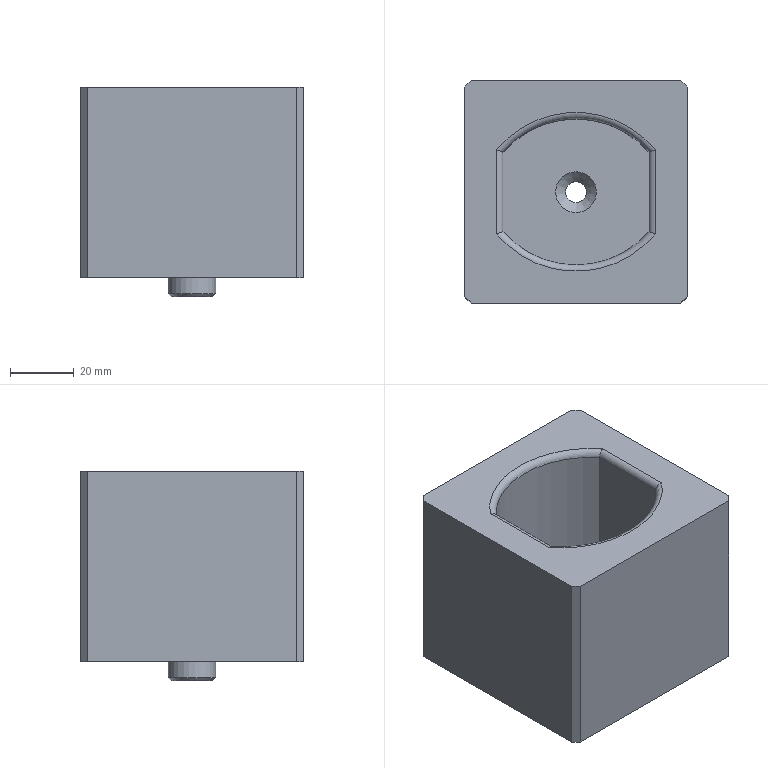NC program | NX | posted with a generic post | part box 70 x 70 x 66 mm
Lines 6381 to 7171 of 8582:
(ZLEVEL_PROFILE_COPY_1_COPY_COPY , TOOL : D6R3)
N12724 T23 M6
N12726 G54
N12728 G17 G0 G90 X-1.4 Y24.719 S7500 M3
N12730 G43 Z30. H23
N12732 Z1.4
N12734 G94 G1 X-3.287 Y24.591 Z1.301 F1000.
N12736 X-5.461 Y24.292 Z1.186
N12738 X-7.61 Y23.847 Z1.071
N12740 X-9.723 Y23.256 Z0.956
N12742 X-11.792 Y22.522 Z0.841
N12744 X-13.805 Y21.649 Z0.726
N12746 X-15.755 Y20.641 Z0.611
N12748 X-17.631 Y19.503 Z0.496
N12750 X-19.425 Y18.239 Z0.381
N12752 X-21.129 Y16.856 Z0.266
N12754 X-22.735 Y15.361 Z0.151
N12756 X-24.236 Y13.759 Z0.036
N12758 X-24.749 Y13.142 Z-0.006
N12760 Y-13.142 F2500.
N12762 G3 X24.749 Y-13.142 R32.189
N12764 G1 Y13.142
N12766 G3 X-24.749 Y13.142 R32.189
N12768 G1 X-24.714 Y13.035 Z-0.008
N12770 X-24.684 Y12.93 Z-0.01
N12772 X-24.656 Y12.824 Z-0.012
N12774 X-24.63 Y12.718 Z-0.014
N12776 Y-13.099
N12778 G3 X24.63 Y-13.099 R32.07
N12780 G1 Y13.099
N12782 G3 X-24.63 Y13.099 R32.07
N12784 G1 X-24.599 Y12.962 Z-0.016
N12786 X-24.57 Y12.826 Z-0.018
N12788 X-24.544 Y12.69 Z-0.021
N12790 X-24.518 Y12.553 Z-0.023
N12792 Y-13.059
N12794 G3 X24.518 Y-13.059 R31.959
N12796 G1 Y13.059
N12798 G3 X-24.518 Y13.059 R31.959
N12800 G1 X-24.489 Y12.893 Z-0.026
N12802 X-24.462 Y12.727 Z-0.029
N12804 X-24.436 Y12.561 Z-0.032
N12806 X-24.411 Y12.395 Z-0.035
N12808 Y-13.02
N12810 G3 X24.411 Y-13.02 R31.851
N12812 G1 Y13.02
N12814 G3 X-24.411 Y13.02 R31.851
N12816 G1 X-24.392 Y12.891 Z-0.037
N12818 X-24.374 Y12.762 Z-0.039
N12820 X-24.356 Y12.633 Z-0.042
N12822 X-24.339 Y12.504 Z-0.044
N12824 X-24.323 Y12.375 Z-0.046
N12826 X-24.306 Y12.246 Z-0.048
N12828 Y-12.982
N12830 G3 X24.306 Y-12.982 R31.747
N12832 G1 Y12.982
N12834 G3 X-24.306 Y12.982 R31.747
N12836 G1 X-24.288 Y12.833 Z-0.051
N12838 X-24.27 Y12.684 Z-0.054
N12840 X-24.253 Y12.535 Z-0.056
N12842 X-24.236 Y12.387 Z-0.059
N12844 X-24.219 Y12.238 Z-0.061
N12846 X-24.203 Y12.089 Z-0.064
N12848 Y-12.944
N12850 G3 X24.203 Y-12.944 R31.644
N12852 G1 Y12.944
N12854 G3 X-24.203 Y12.944 R31.644
N12856 G1 X-24.185 Y12.777 Z-0.067
N12858 X-24.168 Y12.61 Z-0.07
N12860 X-24.151 Y12.443 Z-0.073
N12862 X-24.134 Y12.276 Z-0.076
N12864 X-24.118 Y12.109 Z-0.078
N12866 X-24.102 Y11.943 Z-0.081
N12868 Y-12.907
N12870 G3 X24.102 Y-12.907 R31.542
N12872 G1 Y12.907
N12874 G3 X-24.102 Y12.907 R31.542
N12876 G1 X-24.088 Y12.767 Z-0.084
N12878 X-24.075 Y12.628 Z-0.086
N12880 X-24.062 Y12.488 Z-0.089
N12882 X-24.05 Y12.349 Z-0.091
N12884 X-24.037 Y12.209 Z-0.094
N12886 X-24.025 Y12.07 Z-0.096
N12888 X-24.013 Y11.93 Z-0.098
N12890 X-24.001 Y11.791 Z-0.101
N12892 Y-12.87
N12894 G3 X24.001 Y-12.87 R31.441
N12896 G1 Y12.87
N12898 G3 X-24.001 Y12.87 R31.441
N12900 G1 X-23.988 Y12.716 Z-0.104
N12902 X-23.975 Y12.563 Z-0.106
N12904 X-23.962 Y12.409 Z-0.109
N12906 X-23.95 Y12.255 Z-0.112
N12908 X-23.937 Y12.101 Z-0.114
N12910 X-23.925 Y11.948 Z-0.117
N12912 X-23.913 Y11.794 Z-0.12
N12914 X-23.901 Y11.64 Z-0.122
N12916 Y-12.833
N12918 G3 X23.901 Y-12.833 R31.341
N12920 G1 Y12.833
N12922 G3 X-23.901 Y12.833 R31.341
N12924 G1 X-23.888 Y12.666 Z-0.125
N12926 X-23.875 Y12.498 Z-0.128
N12928 X-23.863 Y12.331 Z-0.131
N12930 X-23.85 Y12.163 Z-0.134
N12932 X-23.838 Y11.995 Z-0.137
N12934 X-23.826 Y11.828 Z-0.14
N12936 X-23.814 Y11.66 Z-0.143
N12938 X-23.802 Y11.493 Z-0.146
N12940 Y-12.797
N12942 G3 X23.802 Y-12.797 R31.242
N12944 G1 Y12.797
N12946 G3 X-23.802 Y12.797 R31.242
N12948 G1 X-23.791 Y12.652 Z-0.148
N12950 X-23.781 Y12.507 Z-0.151
N12952 X-23.771 Y12.362 Z-0.153
N12954 X-23.761 Y12.217 Z-0.156
N12956 X-23.751 Y12.072 Z-0.158
N12958 X-23.742 Y11.927 Z-0.161
N12960 X-23.732 Y11.782 Z-0.163
N12962 X-23.722 Y11.637 Z-0.166
N12964 X-23.713 Y11.492 Z-0.169
N12966 X-23.703 Y11.347 Z-0.171
N12968 Y-12.761
N12970 G3 X23.703 Y-12.761 R31.144
N12972 G1 Y12.761
N12974 G3 X-23.703 Y12.761 R31.144
N12976 G1 X-23.693 Y12.605 Z-0.174
N12978 X-23.683 Y12.448 Z-0.176
N12980 X-23.673 Y12.292 Z-0.179
N12982 X-23.663 Y12.136 Z-0.182
N12984 X-23.654 Y11.98 Z-0.185
N12986 X-23.644 Y11.824 Z-0.187
N12988 X-23.634 Y11.667 Z-0.19
N12990 X-23.625 Y11.511 Z-0.193
N12992 X-23.615 Y11.355 Z-0.196
N12994 X-23.606 Y11.199 Z-0.198
N12996 Y-12.725
N12998 G3 X23.606 Y-12.725 R31.046
N13000 G1 Y12.725
N13002 G3 X-23.606 Y12.725 R31.046
N13004 G1 X-23.596 Y12.558 Z-0.201
N13006 X-23.586 Y12.39 Z-0.204
N13008 X-23.576 Y12.223 Z-0.207
N13010 X-23.566 Y12.056 Z-0.21
N13012 X-23.557 Y11.889 Z-0.213
N13014 X-23.547 Y11.722 Z-0.216
N13016 X-23.537 Y11.554 Z-0.219
N13018 X-23.528 Y11.387 Z-0.222
N13020 X-23.518 Y11.22 Z-0.225
N13022 X-23.509 Y11.053 Z-0.227
N13024 Y-12.689
N13026 G3 X23.509 Y-12.689 R30.949
N13028 G1 Y12.689
N13030 G3 X-23.509 Y12.689 R30.949
N13032 G1 X-23.501 Y12.541 Z-0.23
N13034 X-23.492 Y12.392 Z-0.233
N13036 X-23.484 Y12.244 Z-0.235
N13038 X-23.476 Y12.095 Z-0.238
N13040 X-23.468 Y11.947 Z-0.24
N13042 X-23.46 Y11.799 Z-0.243
N13044 X-23.452 Y11.65 Z-0.246
N13046 X-23.444 Y11.502 Z-0.248
N13048 X-23.436 Y11.354 Z-0.251
N13050 X-23.428 Y11.205 Z-0.253
N13052 X-23.421 Y11.057 Z-0.256
N13054 X-23.413 Y10.908 Z-0.259
N13056 Y-12.653
N13058 G3 X23.413 Y-12.653 R30.853
N13060 G1 Y12.653
N13062 G3 X-23.413 Y12.653 R30.853
N13064 G1 X-23.405 Y12.496 Z-0.261
N13066 X-23.397 Y12.338 Z-0.264
N13068 X-23.388 Y12.181 Z-0.267
N13070 X-23.38 Y12.023 Z-0.27
N13072 X-23.372 Y11.866 Z-0.272
N13074 X-23.364 Y11.708 Z-0.275
N13076 X-23.357 Y11.551 Z-0.278
N13078 X-23.349 Y11.393 Z-0.281
N13080 X-23.341 Y11.236 Z-0.283
N13082 X-23.333 Y11.078 Z-0.286
N13084 X-23.325 Y10.921 Z-0.289
N13086 X-23.318 Y10.763 Z-0.292
N13088 Y-12.618
N13090 G3 X23.318 Y-12.618 R30.758
N13092 G1 Y12.618
N13094 G3 X-23.318 Y12.618 R30.758
N13096 G1 X-23.309 Y12.452 Z-0.294
N13098 X-23.301 Y12.285 Z-0.297
N13100 X-23.293 Y12.119 Z-0.3
N13102 X-23.285 Y11.952 Z-0.303
N13104 X-23.277 Y11.786 Z-0.306
N13106 X-23.27 Y11.619 Z-0.309
N13108 X-23.262 Y11.453 Z-0.312
N13110 X-23.254 Y11.286 Z-0.315
N13112 X-23.246 Y11.12 Z-0.318
N13114 X-23.238 Y10.954 Z-0.321
N13116 X-23.231 Y10.787 Z-0.324
N13118 X-23.223 Y10.621 Z-0.326
N13120 Y-12.583
N13122 G3 X23.223 Y-12.583 R30.663
N13124 G1 Y12.583
N13126 G3 X-23.223 Y12.583 R30.663
N13128 G1 X-23.216 Y12.433 Z-0.329
N13130 X-23.209 Y12.282 Z-0.332
N13132 X-23.202 Y12.132 Z-0.334
N13134 X-23.196 Y11.982 Z-0.337
N13136 X-23.189 Y11.831 Z-0.34
N13138 X-23.182 Y11.681 Z-0.342
N13140 X-23.175 Y11.531 Z-0.345
N13142 X-23.169 Y11.38 Z-0.347
N13144 X-23.162 Y11.23 Z-0.35
N13146 X-23.155 Y11.08 Z-0.353
N13148 X-23.149 Y10.93 Z-0.355
N13150 X-23.142 Y10.779 Z-0.358
N13152 X-23.136 Y10.629 Z-0.361
N13154 X-23.129 Y10.479 Z-0.363
N13156 Y-12.548
N13158 G3 X23.129 Y-12.548 R30.57
N13160 G1 Y12.548
N13162 G3 X-23.129 Y12.548 R30.57
N13164 G1 X-23.122 Y12.39 Z-0.366
N13166 X-23.116 Y12.232 Z-0.369
N13168 X-23.109 Y12.075 Z-0.371
N13170 X-23.102 Y11.917 Z-0.374
N13172 X-23.095 Y11.759 Z-0.377
N13174 X-23.089 Y11.601 Z-0.38
N13176 X-23.082 Y11.443 Z-0.382
N13178 X-23.075 Y11.285 Z-0.385
N13180 X-23.069 Y11.127 Z-0.388
N13182 X-23.062 Y10.969 Z-0.391
N13184 X-23.056 Y10.811 Z-0.393
N13186 X-23.049 Y10.654 Z-0.396
N13188 X-23.043 Y10.496 Z-0.399
N13190 X-23.036 Y10.338 Z-0.402
N13192 Y-12.514
N13194 G3 X23.036 Y-12.514 R30.477
N13196 G1 Y12.514
N13198 G3 X-23.036 Y12.514 R30.477
N13200 G1 X-23.03 Y12.348 Z-0.405
N13202 X-23.023 Y12.183 Z-0.408
N13204 X-23.016 Y12.017 Z-0.41
N13206 X-23.009 Y11.852 Z-0.413
N13208 X-23.003 Y11.686 Z-0.416
N13210 X-22.996 Y11.521 Z-0.419
N13212 X-22.99 Y11.356 Z-0.422
N13214 X-22.983 Y11.19 Z-0.425
N13216 X-22.977 Y11.025 Z-0.428
N13218 X-22.97 Y10.859 Z-0.431
N13220 X-22.964 Y10.694 Z-0.434
N13222 X-22.957 Y10.529 Z-0.436
N13224 X-22.951 Y10.363 Z-0.439
N13226 X-22.944 Y10.198 Z-0.442
N13228 Y-12.479
N13230 G3 X22.944 Y-12.479 R30.385
N13232 G1 Y12.479
N13234 G3 X-22.944 Y12.479 R30.385
N13236 G1 X-22.938 Y12.306 Z-0.445
N13238 X-22.931 Y12.133 Z-0.448
N13240 X-22.924 Y11.961 Z-0.451
N13242 X-22.918 Y11.788 Z-0.454
N13244 X-22.911 Y11.615 Z-0.457
N13246 X-22.905 Y11.442 Z-0.46
N13248 X-22.898 Y11.269 Z-0.463
N13250 X-22.892 Y11.096 Z-0.466
N13252 X-22.885 Y10.923 Z-0.469
N13254 X-22.879 Y10.75 Z-0.472
N13256 X-22.872 Y10.578 Z-0.475
N13258 X-22.866 Y10.405 Z-0.478
N13260 X-22.859 Y10.232 Z-0.481
N13262 X-22.853 Y10.059 Z-0.484
N13264 Y-12.445
N13266 G3 X22.853 Y-12.445 R30.294
N13268 G1 Y12.445
N13270 G3 X-22.853 Y12.445 R30.294
N13272 G1 X-22.847 Y12.287 Z-0.487
N13274 X-22.841 Y12.13 Z-0.49
N13276 X-22.836 Y11.972 Z-0.493
N13278 X-22.83 Y11.814 Z-0.495
N13280 X-22.824 Y11.657 Z-0.498
N13282 X-22.819 Y11.499 Z-0.501
N13284 X-22.813 Y11.341 Z-0.504
N13286 X-22.807 Y11.184 Z-0.506
N13288 X-22.802 Y11.026 Z-0.509
N13290 X-22.796 Y10.868 Z-0.512
N13292 X-22.79 Y10.711 Z-0.515
N13294 X-22.785 Y10.553 Z-0.517
N13296 X-22.779 Y10.395 Z-0.52
N13298 X-22.774 Y10.238 Z-0.523
N13300 X-22.768 Y10.08 Z-0.526
N13302 X-22.763 Y9.922 Z-0.528
N13304 Y-12.411
N13306 G3 X22.763 Y-12.411 R30.203
N13308 G1 Y12.411
N13310 G3 X-22.763 Y12.411 R30.203
N13312 G1 X-22.757 Y12.247 Z-0.531
N13314 X-22.751 Y12.083 Z-0.534
N13316 X-22.746 Y11.919 Z-0.537
N13318 X-22.74 Y11.755 Z-0.54
N13320 X-22.734 Y11.591 Z-0.543
N13322 X-22.729 Y11.426 Z-0.546
N13324 X-22.723 Y11.262 Z-0.549
N13326 X-22.718 Y11.098 Z-0.551
N13328 X-22.712 Y10.934 Z-0.554
N13330 X-22.706 Y10.77 Z-0.557
N13332 X-22.701 Y10.606 Z-0.56
N13334 X-22.695 Y10.442 Z-0.563
N13336 X-22.69 Y10.277 Z-0.566
N13338 X-22.684 Y10.113 Z-0.569
N13340 X-22.679 Y9.949 Z-0.571
N13342 X-22.673 Y9.785 Z-0.574
N13344 Y-12.378
N13346 G3 X22.673 Y-12.378 R30.114
N13348 G1 Y12.378
N13350 G3 X-22.673 Y12.378 R30.114
N13352 G1 X-22.668 Y12.207 Z-0.577
N13354 X-22.662 Y12.037 Z-0.58
N13356 X-22.656 Y11.866 Z-0.583
N13358 X-22.651 Y11.696 Z-0.586
N13360 X-22.645 Y11.526 Z-0.589
N13362 X-22.64 Y11.355 Z-0.592
N13364 X-22.634 Y11.185 Z-0.595
N13366 X-22.629 Y11.014 Z-0.598
N13368 X-22.623 Y10.844 Z-0.601
N13370 X-22.618 Y10.673 Z-0.604
N13372 X-22.612 Y10.503 Z-0.607
N13374 X-22.607 Y10.332 Z-0.61
N13376 X-22.601 Y10.162 Z-0.613
N13378 X-22.596 Y9.992 Z-0.616
N13380 X-22.59 Y9.821 Z-0.619
N13382 X-22.585 Y9.651 Z-0.622
N13384 Y-12.345
N13386 G3 X22.585 Y-12.345 R30.025
N13388 G1 Y12.345
N13390 G3 X-22.585 Y12.345 R30.025
N13392 G1 X-22.58 Y12.187 Z-0.625
N13394 X-22.575 Y12.03 Z-0.627
N13396 X-22.57 Y11.873 Z-0.63
N13398 X-22.565 Y11.716 Z-0.633
N13400 X-22.56 Y11.559 Z-0.636
N13402 X-22.555 Y11.402 Z-0.638
N13404 X-22.551 Y11.245 Z-0.641
N13406 X-22.546 Y11.088 Z-0.644
N13408 X-22.541 Y10.931 Z-0.647
N13410 X-22.536 Y10.774 Z-0.649
N13412 X-22.531 Y10.617 Z-0.652
N13414 X-22.526 Y10.46 Z-0.655
N13416 X-22.521 Y10.303 Z-0.658
N13418 X-22.517 Y10.146 Z-0.66
N13420 X-22.512 Y9.988 Z-0.663
N13422 X-22.507 Y9.831 Z-0.666
N13424 X-22.502 Y9.674 Z-0.669
N13426 X-22.498 Y9.517 Z-0.671
N13428 Y-12.312
N13430 G3 X22.498 Y-12.312 R29.938
N13432 G1 Y12.312
N13434 G3 X-22.498 Y12.312 R29.938
N13436 G1 X-22.493 Y12.149 Z-0.674
N13438 X-22.488 Y11.986 Z-0.677
N13440 X-22.483 Y11.824 Z-0.68
N13442 X-22.478 Y11.661 Z-0.683
N13444 X-22.473 Y11.499 Z-0.685
N13446 X-22.468 Y11.336 Z-0.688
N13448 X-22.464 Y11.174 Z-0.691
N13450 X-22.459 Y11.011 Z-0.694
N13452 X-22.454 Y10.848 Z-0.697
N13454 X-22.449 Y10.686 Z-0.7
N13456 X-22.444 Y10.523 Z-0.702
N13458 X-22.44 Y10.361 Z-0.705
N13460 X-22.435 Y10.198 Z-0.708
N13462 X-22.43 Y10.035 Z-0.711
N13464 X-22.425 Y9.873 Z-0.714
N13466 X-22.421 Y9.71 Z-0.717
N13468 X-22.416 Y9.548 Z-0.719
N13470 X-22.411 Y9.385 Z-0.722
N13472 Y-12.279
N13474 G3 X22.411 Y-12.279 R29.852
N13476 G1 Y12.279
N13478 G3 X-22.411 Y12.279 R29.852
N13480 G1 X-22.406 Y12.111 Z-0.725
N13482 X-22.402 Y11.943 Z-0.728
N13484 X-22.397 Y11.775 Z-0.731
N13486 X-22.392 Y11.607 Z-0.734
N13488 X-22.387 Y11.439 Z-0.737
N13490 X-22.382 Y11.271 Z-0.74
N13492 X-22.378 Y11.103 Z-0.743
N13494 X-22.373 Y10.935 Z-0.746
N13496 X-22.368 Y10.767 Z-0.749
N13498 X-22.363 Y10.599 Z-0.752
N13500 X-22.359 Y10.431 Z-0.755
N13502 X-22.354 Y10.263 Z-0.758
N13504 X-22.349 Y10.095 Z-0.76
N13506 X-22.345 Y9.927 Z-0.763
N13508 X-22.34 Y9.759 Z-0.766
N13510 X-22.335 Y9.591 Z-0.769
N13512 X-22.331 Y9.423 Z-0.772
N13514 X-22.326 Y9.255 Z-0.775
N13516 Y-12.247
N13518 G3 X22.326 Y-12.247 R29.766
N13520 G1 Y12.247
N13522 G3 X-22.326 Y12.247 R29.766
N13524 G1 X-22.322 Y12.091 Z-0.778
N13526 X-22.317 Y11.935 Z-0.781
N13528 X-22.313 Y11.779 Z-0.783
N13530 X-22.309 Y11.623 Z-0.786
N13532 X-22.305 Y11.467 Z-0.789
N13534 X-22.3 Y11.311 Z-0.791
N13536 X-22.296 Y11.155 Z-0.794
N13538 X-22.292 Y10.999 Z-0.797
N13540 X-22.288 Y10.843 Z-0.8
N13542 X-22.283 Y10.686 Z-0.802
N13544 X-22.279 Y10.53 Z-0.805
N13546 X-22.275 Y10.374 Z-0.808
N13548 X-22.271 Y10.218 Z-0.811
N13550 X-22.267 Y10.062 Z-0.813
N13552 X-22.262 Y9.906 Z-0.816
N13554 X-22.258 Y9.75 Z-0.819
N13556 X-22.254 Y9.594 Z-0.821
N13558 X-22.25 Y9.438 Z-0.824
N13560 X-22.246 Y9.282 Z-0.827
N13562 X-22.242 Y9.126 Z-0.83
N13564 Y-12.215
N13566 G3 X22.242 Y-12.215 R29.682
N13568 G1 Y12.215
N13570 G3 X-22.242 Y12.215 R29.682
N13572 G1 X-22.238 Y12.054 Z-0.832
N13574 X-22.233 Y11.893 Z-0.835
N13576 X-22.229 Y11.733 Z-0.838
N13578 X-22.225 Y11.572 Z-0.841
N13580 X-22.221 Y11.411 Z-0.844
N13582 X-22.216 Y11.25 Z-0.846
N13584 X-22.212 Y11.089 Z-0.849
N13586 X-22.208 Y10.928 Z-0.852
N13588 X-22.204 Y10.768 Z-0.855
N13590 X-22.2 Y10.607 Z-0.858
N13592 X-22.196 Y10.446 Z-0.86
N13594 X-22.192 Y10.285 Z-0.863
N13596 X-22.187 Y10.124 Z-0.866
N13598 X-22.183 Y9.963 Z-0.869
N13600 X-22.179 Y9.803 Z-0.872
N13602 X-22.175 Y9.642 Z-0.875
N13604 X-22.171 Y9.481 Z-0.877
N13606 X-22.167 Y9.32 Z-0.88
N13608 X-22.163 Y9.159 Z-0.883
N13610 X-22.159 Y8.998 Z-0.886
N13612 Y-12.184
N13614 G3 X22.159 Y-12.184 R29.599
N13616 G1 Y12.184
N13618 G3 X-22.159 Y12.184 R29.599
N13620 G1 X-22.155 Y12.018 Z-0.889
N13622 X-22.15 Y11.853 Z-0.892
N13624 X-22.146 Y11.687 Z-0.894
N13626 X-22.142 Y11.521 Z-0.897
N13628 X-22.138 Y11.356 Z-0.9
N13630 X-22.134 Y11.19 Z-0.903
N13632 X-22.13 Y11.025 Z-0.906
N13634 X-22.126 Y10.859 Z-0.909
N13636 X-22.121 Y10.694 Z-0.912
N13638 X-22.117 Y10.528 Z-0.915
N13640 X-22.113 Y10.363 Z-0.918
N13642 X-22.109 Y10.197 Z-0.92
N13644 X-22.105 Y10.032 Z-0.923
N13646 X-22.101 Y9.866 Z-0.926
N13648 X-22.097 Y9.701 Z-0.929
N13650 X-22.093 Y9.535 Z-0.932
N13652 X-22.089 Y9.369 Z-0.935
N13654 X-22.085 Y9.204 Z-0.938
N13656 X-22.081 Y9.038 Z-0.941
N13658 X-22.077 Y8.873 Z-0.944
N13660 Y-12.152
N13662 G3 X22.077 Y-12.152 R29.517
N13664 G1 Y12.152
N13666 G3 X-22.077 Y12.152 R29.517
N13668 G1 X-22.073 Y11.982 Z-0.946
N13670 X-22.069 Y11.812 Z-0.949
N13672 X-22.064 Y11.642 Z-0.952
N13674 X-22.06 Y11.472 Z-0.955
N13676 X-22.056 Y11.302 Z-0.958
N13678 X-22.052 Y11.131 Z-0.961
N13680 X-22.048 Y10.961 Z-0.964
N13682 X-22.044 Y10.791 Z-0.967
N13684 X-22.04 Y10.621 Z-0.97
N13686 X-22.036 Y10.451 Z-0.973
N13688 X-22.032 Y10.281 Z-0.976
N13690 X-22.028 Y10.11 Z-0.979
N13692 X-22.024 Y9.94 Z-0.982
N13694 X-22.02 Y9.77 Z-0.985
N13696 X-22.016 Y9.6 Z-0.988
N13698 X-22.012 Y9.43 Z-0.991
N13700 X-22.008 Y9.26 Z-0.994
N13702 X-22.004 Y9.089 Z-0.997
N13704 X-22. Y8.919 Z-1.
N13706 X-21.996 Y8.749 Z-1.003
N13708 Y-12.122
N13710 G3 X21.996 Y-12.122 R29.437
N13712 G1 Y12.122
N13714 G3 X-21.996 Y12.122 R29.437
N13716 G1 X-21.992 Y11.963 Z-1.006
N13718 X-21.989 Y11.804 Z-1.008
N13720 X-21.985 Y11.645 Z-1.011
N13722 X-21.981 Y11.486 Z-1.014
N13724 X-21.978 Y11.328 Z-1.017
N13726 X-21.974 Y11.169 Z-1.02
N13728 X-21.97 Y11.01 Z-1.022
N13730 X-21.967 Y10.851 Z-1.025
N13732 X-21.963 Y10.692 Z-1.028
N13734 X-21.96 Y10.533 Z-1.031
N13736 X-21.956 Y10.374 Z-1.033
N13738 X-21.952 Y10.215 Z-1.036
N13740 X-21.949 Y10.057 Z-1.039
N13742 X-21.945 Y9.898 Z-1.042
N13744 X-21.942 Y9.739 Z-1.045
N13746 X-21.938 Y9.58 Z-1.047
N13748 X-21.934 Y9.421 Z-1.05
N13750 X-21.931 Y9.262 Z-1.053
N13752 X-21.927 Y9.103 Z-1.056
N13754 X-21.924 Y8.945 Z-1.058
N13756 X-21.92 Y8.786 Z-1.061
N13758 X-21.917 Y8.627 Z-1.064
N13760 Y-12.092
N13762 G3 X21.917 Y-12.092 R29.357
N13764 G1 Y12.092
N13766 G3 X-21.917 Y12.092 R29.357
N13768 G1 X-21.913 Y11.929 Z-1.067
N13770 X-21.909 Y11.766 Z-1.07
N13772 X-21.906 Y11.603 Z-1.072
N13774 X-21.902 Y11.44 Z-1.075
N13776 X-21.899 Y11.277 Z-1.078
N13778 X-21.895 Y11.114 Z-1.081
N13780 X-21.891 Y10.951 Z-1.084
N13782 X-21.888 Y10.788 Z-1.087
N13784 X-21.884 Y10.625 Z-1.09
N13786 X-21.881 Y10.462 Z-1.092
N13788 X-21.877 Y10.299 Z-1.095
N13790 X-21.874 Y10.136 Z-1.098
N13792 X-21.87 Y9.973 Z-1.101
N13794 X-21.866 Y9.81 Z-1.104
N13796 X-21.863 Y9.647 Z-1.107
N13798 X-21.859 Y9.484 Z-1.109
N13800 X-21.856 Y9.321 Z-1.112
N13802 X-21.852 Y9.158 Z-1.115
N13804 X-21.849 Y8.996 Z-1.118
N13806 X-21.845 Y8.833 Z-1.121
N13808 X-21.842 Y8.67 Z-1.124
N13810 X-21.838 Y8.507 Z-1.127
N13812 Y-12.062
N13814 G3 X21.838 Y-12.062 R29.279
N13816 G1 Y12.062
N13818 G3 X-21.838 Y12.062 R29.279
N13820 G1 X-21.835 Y11.895 Z-1.129
N13822 X-21.831 Y11.728 Z-1.132
N13824 X-21.828 Y11.561 Z-1.135
N13826 X-21.824 Y11.394 Z-1.138
N13828 X-21.821 Y11.227 Z-1.141
N13830 X-21.817 Y11.06 Z-1.144
N13832 X-21.814 Y10.893 Z-1.147
N13834 X-21.81 Y10.726 Z-1.15
N13836 X-21.806 Y10.559 Z-1.153
N13838 X-21.803 Y10.392 Z-1.156
N13840 X-21.799 Y10.225 Z-1.159
N13842 X-21.796 Y10.058 Z-1.161
N13844 X-21.792 Y9.891 Z-1.164
N13846 X-21.789 Y9.724 Z-1.167
N13848 X-21.786 Y9.557 Z-1.17
N13850 X-21.782 Y9.39 Z-1.173
N13852 X-21.779 Y9.223 Z-1.176
N13854 X-21.775 Y9.056 Z-1.179
N13856 X-21.772 Y8.889 Z-1.182
N13858 X-21.768 Y8.722 Z-1.185
N13860 X-21.765 Y8.555 Z-1.188
N13862 X-21.761 Y8.388 Z-1.191
N13864 Y-12.032
N13866 G3 X21.761 Y-12.032 R29.202
N13868 G1 Y12.032
N13870 G3 X-21.761 Y12.032 R29.202
N13872 G1 X-21.758 Y11.861 Z-1.194
N13874 X-21.754 Y11.69 Z-1.197
N13876 X-21.751 Y11.52 Z-1.2
N13878 X-21.747 Y11.349 Z-1.203
N13880 X-21.744 Y11.178 Z-1.206
N13882 X-21.74 Y11.007 Z-1.209
N13884 X-21.737 Y10.836 Z-1.212
N13886 X-21.733 Y10.665 Z-1.215
N13888 X-21.73 Y10.494 Z-1.217
N13890 X-21.727 Y10.323 Z-1.22
N13892 X-21.723 Y10.152 Z-1.223
N13894 X-21.72 Y9.981 Z-1.226
N13896 X-21.716 Y9.81 Z-1.229
N13898 X-21.713 Y9.639 Z-1.232
N13900 X-21.709 Y9.468 Z-1.235
N13902 X-21.706 Y9.297 Z-1.238
N13904 X-21.703 Y9.126 Z-1.241
N13906 X-21.699 Y8.955 Z-1.244
N13908 X-21.696 Y8.784 Z-1.247
N13910 X-21.692 Y8.613 Z-1.25
N13912 X-21.689 Y8.443 Z-1.253
N13914 X-21.686 Y8.272 Z-1.256
N13916 Y-12.003
N13918 G3 X21.686 Y-12.003 R29.126
N13920 G1 Y12.003
N13922 G3 X-21.686 Y12.003 R29.126
N13924 G1 X-21.683 Y11.843 Z-1.259
N13926 X-21.679 Y11.683 Z-1.262
N13928 X-21.676 Y11.523 Z-1.265
N13930 X-21.673 Y11.362 Z-1.267
N13932 X-21.67 Y11.202 Z-1.27
N13934 X-21.667 Y11.042 Z-1.273
N13936 X-21.664 Y10.881 Z-1.276
N13938 X-21.661 Y10.721 Z-1.279
N13940 X-21.657 Y10.561 Z-1.281
N13942 X-21.654 Y10.401 Z-1.284
N13944 X-21.651 Y10.24 Z-1.287
N13946 X-21.648 Y10.08 Z-1.29
N13948 X-21.645 Y9.92 Z-1.293
N13950 X-21.642 Y9.76 Z-1.295
N13952 X-21.639 Y9.599 Z-1.298
N13954 X-21.636 Y9.439 Z-1.301
N13956 X-21.633 Y9.279 Z-1.304
N13958 X-21.63 Y9.118 Z-1.307
N13960 X-21.627 Y8.958 Z-1.309
N13962 X-21.624 Y8.798 Z-1.312
N13964 X-21.62 Y8.638 Z-1.315
N13966 X-21.617 Y8.477 Z-1.318
N13968 X-21.614 Y8.317 Z-1.321
N13970 X-21.611 Y8.157 Z-1.323
N13972 Y-11.975
N13974 G3 X21.611 Y-11.975 R29.052
N13976 G1 Y11.975
N13978 G3 X-21.611 Y11.975 R29.052
N13980 G1 X-21.608 Y11.811 Z-1.326
N13982 X-21.605 Y11.647 Z-1.329
N13984 X-21.602 Y11.484 Z-1.332
N13986 X-21.599 Y11.32 Z-1.335
N13988 X-21.596 Y11.156 Z-1.338
N13990 X-21.593 Y10.992 Z-1.341
N13992 X-21.59 Y10.828 Z-1.343
N13994 X-21.587 Y10.665 Z-1.346
N13996 X-21.584 Y10.501 Z-1.349
N13998 X-21.581 Y10.337 Z-1.352
N14000 X-21.578 Y10.173 Z-1.355
N14002 X-21.575 Y10.01 Z-1.358
N14004 X-21.571 Y9.846 Z-1.361
N14006 X-21.568 Y9.682 Z-1.363
N14008 X-21.565 Y9.518 Z-1.366
N14010 X-21.562 Y9.354 Z-1.369
N14012 X-21.559 Y9.191 Z-1.372
N14014 X-21.556 Y9.027 Z-1.375
N14016 X-21.553 Y8.863 Z-1.378
N14018 X-21.55 Y8.699 Z-1.381
N14020 X-21.547 Y8.536 Z-1.383
N14022 X-21.544 Y8.372 Z-1.386
N14024 X-21.541 Y8.208 Z-1.389
N14026 X-21.538 Y8.044 Z-1.392
N14028 Y-11.947
N14030 G3 X21.538 Y-11.947 R28.979
N14032 G1 Y11.947
N14034 G3 X-21.538 Y11.947 R28.979
N14036 G1 X-21.535 Y11.78 Z-1.395
N14038 X-21.532 Y11.613 Z-1.398
N14040 X-21.529 Y11.445 Z-1.401
N14042 X-21.526 Y11.278 Z-1.404
N14044 X-21.523 Y11.111 Z-1.407
N14046 X-21.52 Y10.944 Z-1.41
N14048 X-21.517 Y10.776 Z-1.412
N14050 X-21.514 Y10.609 Z-1.415
N14052 X-21.511 Y10.442 Z-1.418
N14054 X-21.508 Y10.275 Z-1.421
N14056 X-21.505 Y10.108 Z-1.424
N14058 X-21.502 Y9.94 Z-1.427
N14060 X-21.499 Y9.773 Z-1.43
N14062 X-21.496 Y9.606 Z-1.433
N14064 X-21.493 Y9.439 Z-1.436
N14066 X-21.49 Y9.271 Z-1.439
N14068 X-21.487 Y9.104 Z-1.442
N14070 X-21.484 Y8.937 Z-1.445
N14072 X-21.482 Y8.77 Z-1.447
N14074 X-21.479 Y8.603 Z-1.45
N14076 X-21.476 Y8.435 Z-1.453
N14078 X-21.473 Y8.268 Z-1.456
N14080 X-21.47 Y8.101 Z-1.459
N14082 X-21.467 Y7.934 Z-1.462
N14084 Y-11.919
N14086 G3 X21.467 Y-11.919 R28.907
N14088 G1 Y11.919
N14090 G3 X-21.467 Y11.919 R28.907
N14092 G1 X-21.464 Y11.749 Z-1.465
N14094 X-21.461 Y11.578 Z-1.468
N14096 X-21.458 Y11.408 Z-1.471
N14098 X-21.455 Y11.237 Z-1.474
N14100 X-21.452 Y11.067 Z-1.477
N14102 X-21.449 Y10.896 Z-1.48
N14104 X-21.446 Y10.725 Z-1.483
N14106 X-21.443 Y10.555 Z-1.486
N14108 X-21.44 Y10.384 Z-1.489
N14110 X-21.437 Y10.214 Z-1.492
N14112 X-21.434 Y10.043 Z-1.495
N14114 X-21.431 Y9.872 Z-1.498
N14116 X-21.429 Y9.702 Z-1.501
N14118 X-21.426 Y9.531 Z-1.504
N14120 X-21.423 Y9.361 Z-1.507
N14122 X-21.42 Y9.19 Z-1.51
N14124 X-21.417 Y9.019 Z-1.513
N14126 X-21.414 Y8.849 Z-1.516
N14128 X-21.411 Y8.678 Z-1.519
N14130 X-21.408 Y8.508 Z-1.522
N14132 X-21.405 Y8.337 Z-1.525
N14134 X-21.402 Y8.166 Z-1.528
N14136 X-21.4 Y7.996 Z-1.531
N14138 X-21.397 Y7.825 Z-1.534
N14140 Y-11.893
N14142 G3 X21.397 Y-11.893 R28.837
N14144 G1 Y11.893
N14146 G3 X-21.397 Y11.893 R28.837
N14148 G1 X-21.394 Y11.732 Z-1.536
N14150 X-21.391 Y11.571 Z-1.539
N14152 X-21.389 Y11.411 Z-1.542
N14154 X-21.386 Y11.25 Z-1.545
N14156 X-21.383 Y11.09 Z-1.548
N14158 X-21.381 Y10.929 Z-1.55
N14160 X-21.378 Y10.769 Z-1.553
N14162 X-21.375 Y10.608 Z-1.556
N14164 X-21.373 Y10.448 Z-1.559
N14166 X-21.37 Y10.287 Z-1.562
N14168 X-21.367 Y10.127 Z-1.564
N14170 X-21.365 Y9.966 Z-1.567
N14172 X-21.362 Y9.806 Z-1.57
N14174 X-21.359 Y9.645 Z-1.573
N14176 X-21.357 Y9.485 Z-1.576
N14178 X-21.354 Y9.324 Z-1.578
N14180 X-21.351 Y9.164 Z-1.581
N14182 X-21.349 Y9.003 Z-1.584
N14184 X-21.346 Y8.843 Z-1.587
N14186 X-21.344 Y8.682 Z-1.59
N14188 X-21.341 Y8.522 Z-1.592
N14190 X-21.338 Y8.361 Z-1.595
N14192 X-21.336 Y8.201 Z-1.598
N14194 X-21.333 Y8.04 Z-1.601
N14196 X-21.331 Y7.88 Z-1.604
N14198 X-21.328 Y7.719 Z-1.606
N14200 Y-11.866
N14202 G3 X21.328 Y-11.866 R28.768
N14204 G1 Y11.866
N14206 G3 X-21.328 Y11.866 R28.768
N14208 G1 X-21.325 Y11.703 Z-1.609
N14210 X-21.323 Y11.539 Z-1.612
N14212 X-21.32 Y11.376 Z-1.615
N14214 X-21.317 Y11.212 Z-1.618
N14216 X-21.315 Y11.048 Z-1.621
N14218 X-21.312 Y10.885 Z-1.624
N14220 X-21.31 Y10.721 Z-1.626
N14222 X-21.307 Y10.558 Z-1.629
N14224 X-21.304 Y10.394 Z-1.632
N14226 X-21.302 Y10.231 Z-1.635
N14228 X-21.299 Y10.067 Z-1.638
N14230 X-21.297 Y9.904 Z-1.641
N14232 X-21.294 Y9.74 Z-1.644
N14234 X-21.291 Y9.577 Z-1.646
N14236 X-21.289 Y9.413 Z-1.649
N14238 X-21.286 Y9.25 Z-1.652
N14240 X-21.284 Y9.086 Z-1.655
N14242 X-21.281 Y8.923 Z-1.658
N14244 X-21.279 Y8.759 Z-1.661
N14246 X-21.276 Y8.596 Z-1.663
N14248 X-21.274 Y8.432 Z-1.666
N14250 X-21.271 Y8.269 Z-1.669
N14252 X-21.268 Y8.105 Z-1.672
N14254 X-21.266 Y7.942 Z-1.675
N14256 X-21.263 Y7.778 Z-1.678
N14258 X-21.261 Y7.615 Z-1.681
N14260 Y-11.84
N14262 G3 X21.261 Y-11.84 R28.701
N14264 G1 Y11.84
N14266 G3 X-21.261 Y11.84 R28.701
N14268 G1 X-21.258 Y11.674 Z-1.684
N14270 X-21.256 Y11.507 Z-1.686
N14272 X-21.253 Y11.341 Z-1.689
N14274 X-21.251 Y11.174 Z-1.692
N14276 X-21.248 Y11.008 Z-1.695
N14278 X-21.245 Y10.842 Z-1.698
N14280 X-21.243 Y10.675 Z-1.701
N14282 X-21.24 Y10.509 Z-1.704
N14284 X-21.238 Y10.342 Z-1.707
N14286 X-21.235 Y10.176 Z-1.71
N14288 X-21.233 Y10.009 Z-1.713
N14290 X-21.23 Y9.843 Z-1.715
N14292 X-21.228 Y9.677 Z-1.718
N14294 X-21.225 Y9.51 Z-1.721
N14296 X-21.223 Y9.344 Z-1.724
N14298 X-21.22 Y9.177 Z-1.727